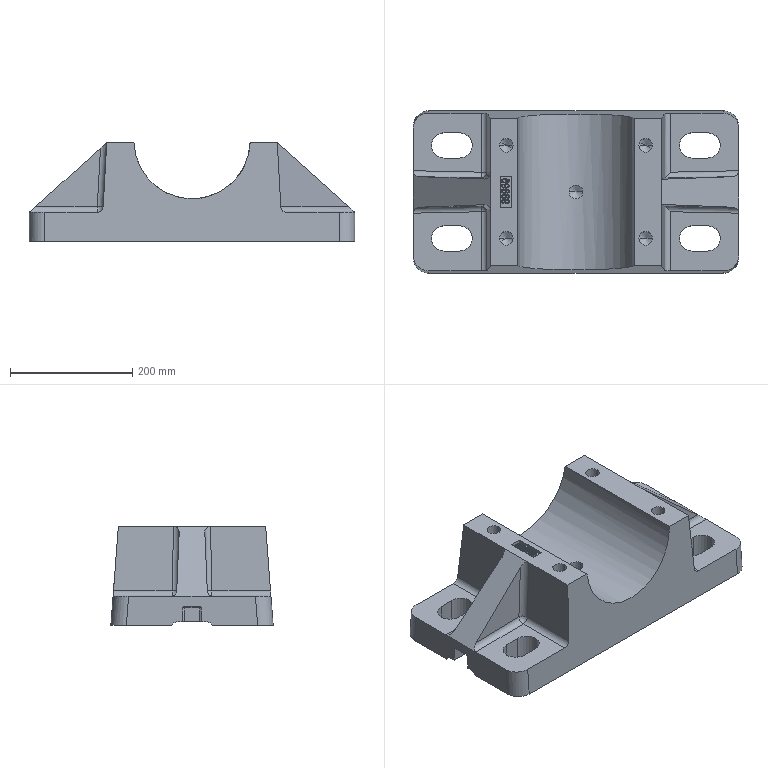Part | SolidWorks | features Cut 6, MirrorPattern 4, Boss 3, Fillet 3, 3DProfileFeature 1, Extrusion 1, HoleWzd 1, RevCut 1 | 1 solid | 192 faces | box 533.4 x 265.974 x 161.862 mm | volume 11273677 mm3 | plane 65 | spline 62 | cylinder 49 | cone 10 | sphere 6 | commonest cylinder face diameters 41.402 x12 6.35 x10 19.05 x10 22.225 x8 50.8 x4 22.631 x2